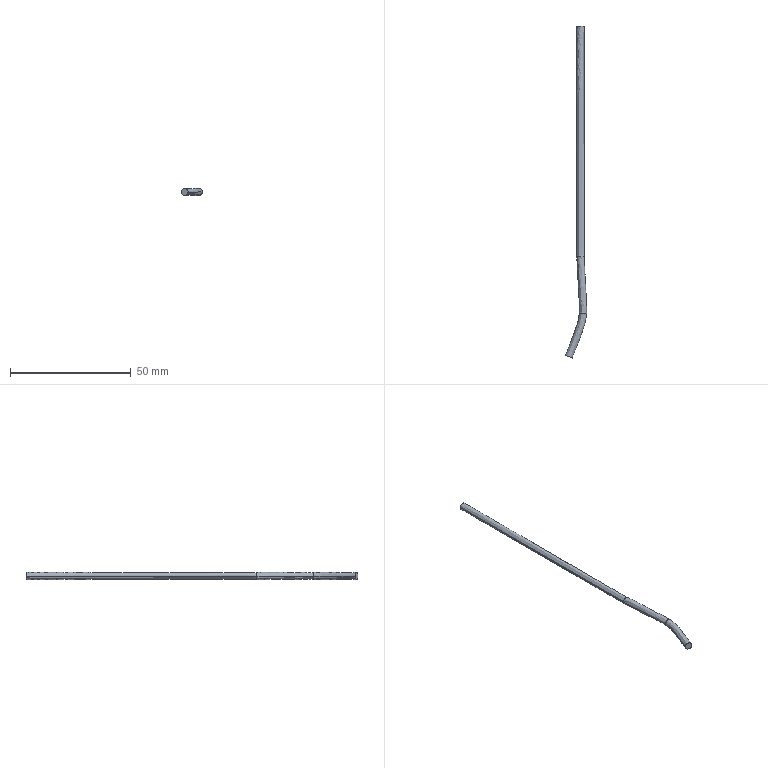Part | NX | features BREP 1 | 1 solid | 8 faces | box 8.835 x 137.527 x 3 mm | volume 975.444 mm3 | spline 6 | plane 2